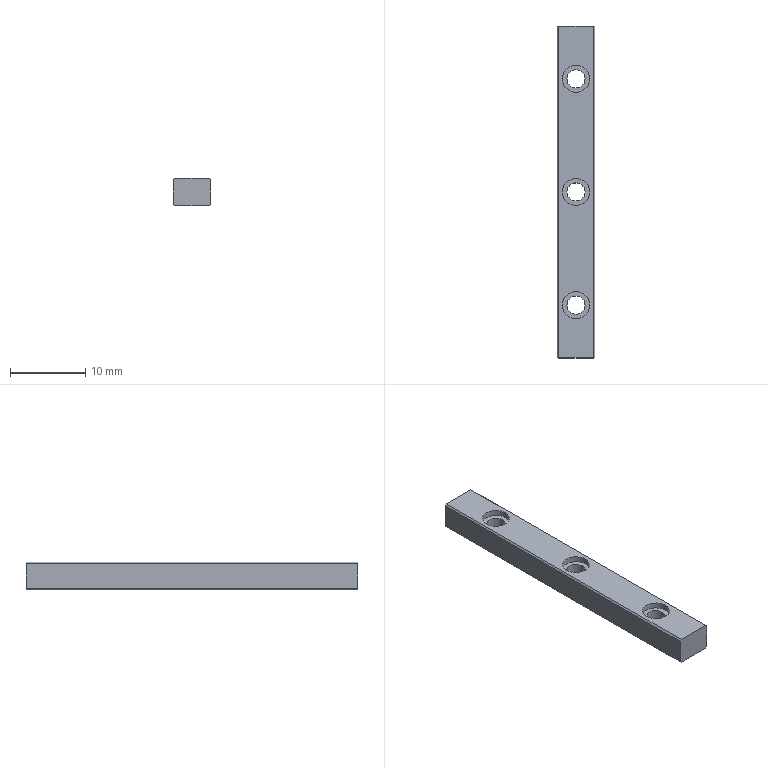Part | SolidWorks | features BaseBody 1 | 1 solid | 25 faces | box 5 x 44 x 3.7 mm | volume 746.693 mm3 | plane 13 | cylinder 12 | commonest cylinder face diameters 2.4 x6 3.6 x6
STEP:
#1=CARTESIAN_POINT('',(13.914,-6.044,0.));
#2=VERTEX_POINT('',#1);
#3=CARTESIAN_POINT('',(11.514,-6.044,0.));
#4=VERTEX_POINT('',#3);
#5=CARTESIAN_POINT('',(12.714,-6.044,0.));
#6=DIRECTION('',(0.,0.,-1.));
#7=DIRECTION('',(1.,0.,0.));
#8=AXIS2_PLACEMENT_3D('',#5,#6,#7);
#9=CIRCLE('',#8,1.2);
#10=EDGE_CURVE('',#2,#4,#9,.T.);
#11=ORIENTED_EDGE('',*,*,#10,.T.);
#12=CARTESIAN_POINT('',(11.514,-6.044,2.9));
#13=VERTEX_POINT('',#12);
#14=CARTESIAN_POINT('',(11.514,-6.044,-48.671));
#15=DIRECTION('',(0.,0.,1.));
#16=VECTOR('',#15,1000.);
#17=LINE('',#14,#16);
#18=EDGE_CURVE('',#4,#13,#17,.T.);
#19=ORIENTED_EDGE('',*,*,#18,.T.);
#20=CARTESIAN_POINT('',(13.914,-6.044,2.9));
#21=VERTEX_POINT('',#20);
#22=CARTESIAN_POINT('',(12.714,-6.044,2.9));
#23=DIRECTION('',(0.,0.,-1.));
#24=DIRECTION('',(1.,0.,0.));
#25=AXIS2_PLACEMENT_3D('',#22,#23,#24);
#26=CIRCLE('',#25,1.2);
#27=EDGE_CURVE('',#21,#13,#26,.T.);
#28=ORIENTED_EDGE('',*,*,#27,.F.);
#29=CARTESIAN_POINT('',(13.914,-6.044,-48.671));
#30=DIRECTION('',(0.,0.,1.));
#31=VECTOR('',#30,1000.);
#32=LINE('',#29,#31);
#33=EDGE_CURVE('',#2,#21,#32,.T.);
#34=ORIENTED_EDGE('',*,*,#33,.F.);
#35=EDGE_LOOP('',(#11,#19,#28,#34));
#36=FACE_OUTER_BOUND('',#35,.T.);
#37=CARTESIAN_POINT('',(12.714,-6.044,-48.671));
#38=DIRECTION('',(0.,0.,1.));
#39=DIRECTION('',(1.,0.,0.));
#40=AXIS2_PLACEMENT_3D('',#37,#38,#39);
#41=CYLINDRICAL_SURFACE('',#40,1.2);
#42=ADVANCED_FACE('',(#36),#41,.F.);
#43=CARTESIAN_POINT('',(13.914,-21.044,0.));
#44=VERTEX_POINT('',#43);
#45=CARTESIAN_POINT('',(11.514,-21.044,0.));
#46=VERTEX_POINT('',#45);
#47=CARTESIAN_POINT('',(12.714,-21.044,0.));
#48=DIRECTION('',(0.,0.,-1.));
#49=DIRECTION('',(1.,0.,0.));
#50=AXIS2_PLACEMENT_3D('',#47,#48,#49);
#51=CIRCLE('',#50,1.2);
#52=EDGE_CURVE('',#44,#46,#51,.T.);
#53=ORIENTED_EDGE('',*,*,#52,.T.);
#54=CARTESIAN_POINT('',(11.514,-21.044,2.9));
#55=VERTEX_POINT('',#54);
#56=CARTESIAN_POINT('',(11.514,-21.044,-48.671));
#57=DIRECTION('',(0.,0.,1.));
#58=VECTOR('',#57,1000.);
#59=LINE('',#56,#58);
#60=EDGE_CURVE('',#46,#55,#59,.T.);
#61=ORIENTED_EDGE('',*,*,#60,.T.);
#62=CARTESIAN_POINT('',(13.914,-21.044,2.9));
#63=VERTEX_POINT('',#62);
#64=CARTESIAN_POINT('',(12.714,-21.044,2.9));
#65=DIRECTION('',(0.,0.,-1.));
#66=DIRECTION('',(1.,0.,0.));
#67=AXIS2_PLACEMENT_3D('',#64,#65,#66);
#68=CIRCLE('',#67,1.2);
#69=EDGE_CURVE('',#63,#55,#68,.T.);
#70=ORIENTED_EDGE('',*,*,#69,.F.);
#71=CARTESIAN_POINT('',(13.914,-21.044,-48.671));
#72=DIRECTION('',(0.,0.,1.));
#73=VECTOR('',#72,1000.);
#74=LINE('',#71,#73);
#75=EDGE_CURVE('',#44,#63,#74,.T.);
#76=ORIENTED_EDGE('',*,*,#75,.F.);
#77=EDGE_LOOP('',(#53,#61,#70,#76));
#78=FACE_OUTER_BOUND('',#77,.T.);
#79=CARTESIAN_POINT('',(12.714,-21.044,-48.671));
#80=DIRECTION('',(0.,0.,1.));
#81=DIRECTION('',(1.,0.,0.));
#82=AXIS2_PLACEMENT_3D('',#79,#80,#81);
#83=CYLINDRICAL_SURFACE('',#82,1.2);
#84=ADVANCED_FACE('',(#78),#83,.F.);
#85=CARTESIAN_POINT('',(13.914,-36.044,0.));
#86=VERTEX_POINT('',#85);
#87=CARTESIAN_POINT('',(11.514,-36.044,0.));
#88=VERTEX_POINT('',#87);
#89=CARTESIAN_POINT('',(12.714,-36.044,0.));
#90=DIRECTION('',(0.,0.,-1.));
#91=DIRECTION('',(1.,0.,0.));
#92=AXIS2_PLACEMENT_3D('',#89,#90,#91);
#93=CIRCLE('',#92,1.2);
#94=EDGE_CURVE('',#86,#88,#93,.T.);
#95=ORIENTED_EDGE('',*,*,#94,.T.);
#96=CARTESIAN_POINT('',(11.514,-36.044,2.9));
#97=VERTEX_POINT('',#96);
#98=CARTESIAN_POINT('',(11.514,-36.044,-48.671));
#99=DIRECTION('',(0.,0.,1.));
#100=VECTOR('',#99,1000.);
#101=LINE('',#98,#100);
#102=EDGE_CURVE('',#88,#97,#101,.T.);
#103=ORIENTED_EDGE('',*,*,#102,.T.);
#104=CARTESIAN_POINT('',(13.914,-36.044,2.9));
#105=VERTEX_POINT('',#104);
#106=CARTESIAN_POINT('',(12.714,-36.044,2.9));
#107=DIRECTION('',(0.,0.,-1.));
#108=DIRECTION('',(1.,0.,0.));
#109=AXIS2_PLACEMENT_3D('',#106,#107,#108);
#110=CIRCLE('',#109,1.2);
#111=EDGE_CURVE('',#105,#97,#110,.T.);
#112=ORIENTED_EDGE('',*,*,#111,.F.);
#113=CARTESIAN_POINT('',(13.914,-36.044,-48.671));
#114=DIRECTION('',(0.,0.,1.));
#115=VECTOR('',#114,1000.);
#116=LINE('',#113,#115);
#117=EDGE_CURVE('',#86,#105,#116,.T.);
#118=ORIENTED_EDGE('',*,*,#117,.F.);
#119=EDGE_LOOP('',(#95,#103,#112,#118));
#120=FACE_OUTER_BOUND('',#119,.T.);
#121=CARTESIAN_POINT('',(12.714,-36.044,-48.671));
#122=DIRECTION('',(0.,0.,1.));
#123=DIRECTION('',(1.,0.,0.));
#124=AXIS2_PLACEMENT_3D('',#121,#122,#123);
#125=CYLINDRICAL_SURFACE('',#124,1.2);
#126=ADVANCED_FACE('',(#120),#125,.F.);
#127=CARTESIAN_POINT('',(10.914,-6.044,2.9));
#128=VERTEX_POINT('',#127);
#129=CARTESIAN_POINT('',(14.514,-6.044,2.9));
#130=VERTEX_POINT('',#129);
#131=CARTESIAN_POINT('',(12.714,-6.044,2.9));
#132=DIRECTION('',(0.,0.,1.));
#133=DIRECTION('',(1.,0.,0.));
#134=AXIS2_PLACEMENT_3D('',#131,#132,#133);
#135=CIRCLE('',#134,1.8);
#136=EDGE_CURVE('',#128,#130,#135,.T.);
#137=ORIENTED_EDGE('',*,*,#136,.F.);
#138=CARTESIAN_POINT('',(10.914,-6.044,3.7));
#139=VERTEX_POINT('',#138);
#140=CARTESIAN_POINT('',(10.914,-6.044,3.3));
#141=DIRECTION('',(0.,0.,1.));
#142=VECTOR('',#141,1000.);
#143=LINE('',#140,#142);
#144=EDGE_CURVE('',#128,#139,#143,.T.);
#145=ORIENTED_EDGE('',*,*,#144,.T.);
#146=CARTESIAN_POINT('',(14.514,-6.044,3.7));
#147=VERTEX_POINT('',#146);
#148=CARTESIAN_POINT('',(12.714,-6.044,3.7));
#149=DIRECTION('',(0.,0.,-1.));
#150=DIRECTION('',(1.,0.,0.));
#151=AXIS2_PLACEMENT_3D('',#148,#149,#150);
#152=CIRCLE('',#151,1.8);
#153=EDGE_CURVE('',#147,#139,#152,.T.);
#154=ORIENTED_EDGE('',*,*,#153,.F.);
#155=CARTESIAN_POINT('',(14.514,-6.044,3.3));
#156=DIRECTION('',(0.,0.,1.));
#157=VECTOR('',#156,1000.);
#158=LINE('',#155,#157);
#159=EDGE_CURVE('',#130,#147,#158,.T.);
#160=ORIENTED_EDGE('',*,*,#159,.F.);
#161=EDGE_LOOP('',(#137,#145,#154,#160));
#162=FACE_OUTER_BOUND('',#161,.T.);
#163=CARTESIAN_POINT('',(12.714,-6.044,3.3));
#164=DIRECTION('',(0.,0.,1.));
#165=DIRECTION('',(1.,0.,0.));
#166=AXIS2_PLACEMENT_3D('',#163,#164,#165);
#167=CYLINDRICAL_SURFACE('',#166,1.8);
#168=ADVANCED_FACE('',(#162),#167,.F.);
#169=CARTESIAN_POINT('',(10.914,-21.044,2.9));
#170=VERTEX_POINT('',#169);
#171=CARTESIAN_POINT('',(14.514,-21.044,2.9));
#172=VERTEX_POINT('',#171);
#173=CARTESIAN_POINT('',(12.714,-21.044,2.9));
#174=DIRECTION('',(0.,0.,1.));
#175=DIRECTION('',(1.,0.,0.));
#176=AXIS2_PLACEMENT_3D('',#173,#174,#175);
#177=CIRCLE('',#176,1.8);
#178=EDGE_CURVE('',#170,#172,#177,.T.);
#179=ORIENTED_EDGE('',*,*,#178,.F.);
#180=CARTESIAN_POINT('',(10.914,-21.044,3.7));
#181=VERTEX_POINT('',#180);
#182=CARTESIAN_POINT('',(10.914,-21.044,3.3));
#183=DIRECTION('',(0.,0.,1.));
#184=VECTOR('',#183,1000.);
#185=LINE('',#182,#184);
#186=EDGE_CURVE('',#170,#181,#185,.T.);
#187=ORIENTED_EDGE('',*,*,#186,.T.);
#188=CARTESIAN_POINT('',(14.514,-21.044,3.7));
#189=VERTEX_POINT('',#188);
#190=CARTESIAN_POINT('',(12.714,-21.044,3.7));
#191=DIRECTION('',(0.,0.,-1.));
#192=DIRECTION('',(1.,0.,0.));
#193=AXIS2_PLACEMENT_3D('',#190,#191,#192);
#194=CIRCLE('',#193,1.8);
#195=EDGE_CURVE('',#189,#181,#194,.T.);
#196=ORIENTED_EDGE('',*,*,#195,.F.);
#197=CARTESIAN_POINT('',(14.514,-21.044,3.3));
#198=DIRECTION('',(0.,0.,1.));
#199=VECTOR('',#198,1000.);
#200=LINE('',#197,#199);
#201=EDGE_CURVE('',#172,#189,#200,.T.);
#202=ORIENTED_EDGE('',*,*,#201,.F.);
#203=EDGE_LOOP('',(#179,#187,#196,#202));
#204=FACE_OUTER_BOUND('',#203,.T.);
#205=CARTESIAN_POINT('',(12.714,-21.044,3.3));
#206=DIRECTION('',(0.,0.,1.));
#207=DIRECTION('',(1.,0.,0.));
#208=AXIS2_PLACEMENT_3D('',#205,#206,#207);
#209=CYLINDRICAL_SURFACE('',#208,1.8);
#210=ADVANCED_FACE('',(#204),#209,.F.);
#211=CARTESIAN_POINT('',(10.914,-36.044,2.9));
#212=VERTEX_POINT('',#211);
#213=CARTESIAN_POINT('',(14.514,-36.044,2.9));
#214=VERTEX_POINT('',#213);
#215=CARTESIAN_POINT('',(12.714,-36.044,2.9));
#216=DIRECTION('',(0.,0.,1.));
#217=DIRECTION('',(1.,0.,0.));
#218=AXIS2_PLACEMENT_3D('',#215,#216,#217);
#219=CIRCLE('',#218,1.8);
#220=EDGE_CURVE('',#212,#214,#219,.T.);
#221=ORIENTED_EDGE('',*,*,#220,.F.);
#222=CARTESIAN_POINT('',(10.914,-36.044,3.7));
#223=VERTEX_POINT('',#222);
#224=CARTESIAN_POINT('',(10.914,-36.044,3.3));
#225=DIRECTION('',(0.,0.,1.));
#226=VECTOR('',#225,1000.);
#227=LINE('',#224,#226);
#228=EDGE_CURVE('',#212,#223,#227,.T.);
#229=ORIENTED_EDGE('',*,*,#228,.T.);
#230=CARTESIAN_POINT('',(14.514,-36.044,3.7));
#231=VERTEX_POINT('',#230);
#232=CARTESIAN_POINT('',(12.714,-36.044,3.7));
#233=DIRECTION('',(0.,0.,-1.));
#234=DIRECTION('',(1.,0.,0.));
#235=AXIS2_PLACEMENT_3D('',#232,#233,#234);
#236=CIRCLE('',#235,1.8);
#237=EDGE_CURVE('',#231,#223,#236,.T.);
#238=ORIENTED_EDGE('',*,*,#237,.F.);
#239=CARTESIAN_POINT('',(14.514,-36.044,3.3));
#240=DIRECTION('',(0.,0.,1.));
#241=VECTOR('',#240,1000.);
#242=LINE('',#239,#241);
#243=EDGE_CURVE('',#214,#231,#242,.T.);
#244=ORIENTED_EDGE('',*,*,#243,.F.);
#245=EDGE_LOOP('',(#221,#229,#238,#244));
#246=FACE_OUTER_BOUND('',#245,.T.);
#247=CARTESIAN_POINT('',(12.714,-36.044,3.3));
#248=DIRECTION('',(0.,0.,1.));
#249=DIRECTION('',(1.,0.,0.));
#250=AXIS2_PLACEMENT_3D('',#247,#248,#249);
#251=CYLINDRICAL_SURFACE('',#250,1.8);
#252=ADVANCED_FACE('',(#246),#251,.F.);
#253=ORIENTED_EDGE('',*,*,#10,.F.);
#254=CARTESIAN_POINT('',(12.714,-6.044,0.));
#255=DIRECTION('',(0.,0.,-1.));
#256=DIRECTION('',(1.,0.,0.));
#257=AXIS2_PLACEMENT_3D('',#254,#255,#256);
#258=CIRCLE('',#257,1.2);
#259=EDGE_CURVE('',#4,#2,#258,.T.);
#260=ORIENTED_EDGE('',*,*,#259,.F.);
#261=EDGE_LOOP('',(#253,#260));
#262=FACE_BOUND('',#261,.T.);
#263=ORIENTED_EDGE('',*,*,#52,.F.);
#264=CARTESIAN_POINT('',(12.714,-21.044,0.));
#265=DIRECTION('',(0.,0.,-1.));
#266=DIRECTION('',(1.,0.,0.));
#267=AXIS2_PLACEMENT_3D('',#264,#265,#266);
#268=CIRCLE('',#267,1.2);
#269=EDGE_CURVE('',#46,#44,#268,.T.);
#270=ORIENTED_EDGE('',*,*,#269,.F.);
#271=EDGE_LOOP('',(#263,#270));
#272=FACE_BOUND('',#271,.T.);
#273=ORIENTED_EDGE('',*,*,#94,.F.);
#274=CARTESIAN_POINT('',(12.714,-36.044,0.));
#275=DIRECTION('',(0.,0.,-1.));
#276=DIRECTION('',(1.,0.,0.));
#277=AXIS2_PLACEMENT_3D('',#274,#275,#276);
#278=CIRCLE('',#277,1.2);
#279=EDGE_CURVE('',#88,#86,#278,.T.);
#280=ORIENTED_EDGE('',*,*,#279,.F.);
#281=EDGE_LOOP('',(#273,#280));
#282=FACE_BOUND('',#281,.T.);
#283=CARTESIAN_POINT('',(10.414,-43.044,0.));
#284=VERTEX_POINT('',#283);
#285=CARTESIAN_POINT('',(15.014,-43.044,0.));
#286=VERTEX_POINT('',#285);
#287=CARTESIAN_POINT('',(12.714,-43.044,0.));
#288=DIRECTION('',(1.,0.,0.));
#289=VECTOR('',#288,1000.);
#290=LINE('',#287,#289);
#291=EDGE_CURVE('',#284,#286,#290,.T.);
#292=ORIENTED_EDGE('',*,*,#291,.F.);
#293=CARTESIAN_POINT('',(10.414,0.9558,0.));
#294=VERTEX_POINT('',#293);
#295=CARTESIAN_POINT('',(10.414,-21.044,0.));
#296=DIRECTION('',(0.,-1.,0.));
#297=VECTOR('',#296,1000.);
#298=LINE('',#295,#297);
#299=EDGE_CURVE('',#294,#284,#298,.T.);
#300=ORIENTED_EDGE('',*,*,#299,.F.);
#301=CARTESIAN_POINT('',(15.014,0.9558,0.));
#302=VERTEX_POINT('',#301);
#303=CARTESIAN_POINT('',(12.714,0.9558,0.));
#304=DIRECTION('',(-1.,0.,0.));
#305=VECTOR('',#304,1000.);
#306=LINE('',#303,#305);
#307=EDGE_CURVE('',#302,#294,#306,.T.);
#308=ORIENTED_EDGE('',*,*,#307,.F.);
#309=CARTESIAN_POINT('',(15.014,-21.044,0.));
#310=DIRECTION('',(0.,1.,0.));
#311=VECTOR('',#310,1000.);
#312=LINE('',#309,#311);
#313=EDGE_CURVE('',#286,#302,#312,.T.);
#314=ORIENTED_EDGE('',*,*,#313,.F.);
#315=EDGE_LOOP('',(#292,#300,#308,#314));
#316=FACE_OUTER_BOUND('',#315,.T.);
#317=CARTESIAN_POINT('',(12.714,-21.044,0.));
#318=DIRECTION('',(0.,0.,1.));
#319=DIRECTION('',(1.,0.,0.));
#320=AXIS2_PLACEMENT_3D('',#317,#318,#319);
#321=PLANE('',#320);
#322=ADVANCED_FACE('',(#262,#272,#282,#316),#321,.F.);
#323=ORIENTED_EDGE('',*,*,#18,.F.);
#324=ORIENTED_EDGE('',*,*,#259,.T.);
#325=ORIENTED_EDGE('',*,*,#33,.T.);
#326=CARTESIAN_POINT('',(12.714,-6.044,2.9));
#327=DIRECTION('',(0.,0.,-1.));
#328=DIRECTION('',(1.,0.,0.));
#329=AXIS2_PLACEMENT_3D('',#326,#327,#328);
#330=CIRCLE('',#329,1.2);
#331=EDGE_CURVE('',#13,#21,#330,.T.);
#332=ORIENTED_EDGE('',*,*,#331,.F.);
#333=EDGE_LOOP('',(#323,#324,#325,#332));
#334=FACE_OUTER_BOUND('',#333,.T.);
#335=CARTESIAN_POINT('',(12.714,-6.044,-48.671));
#336=DIRECTION('',(0.,0.,1.));
#337=DIRECTION('',(1.,0.,0.));
#338=AXIS2_PLACEMENT_3D('',#335,#336,#337);
#339=CYLINDRICAL_SURFACE('',#338,1.2);
#340=ADVANCED_FACE('',(#334),#339,.F.);
#341=ORIENTED_EDGE('',*,*,#60,.F.);
#342=ORIENTED_EDGE('',*,*,#269,.T.);
#343=ORIENTED_EDGE('',*,*,#75,.T.);
#344=CARTESIAN_POINT('',(12.714,-21.044,2.9));
#345=DIRECTION('',(0.,0.,-1.));
#346=DIRECTION('',(1.,0.,0.));
#347=AXIS2_PLACEMENT_3D('',#344,#345,#346);
#348=CIRCLE('',#347,1.2);
#349=EDGE_CURVE('',#55,#63,#348,.T.);
#350=ORIENTED_EDGE('',*,*,#349,.F.);
#351=EDGE_LOOP('',(#341,#342,#343,#350));
#352=FACE_OUTER_BOUND('',#351,.T.);
#353=CARTESIAN_POINT('',(12.714,-21.044,-48.671));
#354=DIRECTION('',(0.,0.,1.));
#355=DIRECTION('',(1.,0.,0.));
#356=AXIS2_PLACEMENT_3D('',#353,#354,#355);
#357=CYLINDRICAL_SURFACE('',#356,1.2);
#358=ADVANCED_FACE('',(#352),#357,.F.);
#359=ORIENTED_EDGE('',*,*,#102,.F.);
#360=ORIENTED_EDGE('',*,*,#279,.T.);
#361=ORIENTED_EDGE('',*,*,#117,.T.);
#362=CARTESIAN_POINT('',(12.714,-36.044,2.9));
#363=DIRECTION('',(0.,0.,-1.));
#364=DIRECTION('',(1.,0.,0.));
#365=AXIS2_PLACEMENT_3D('',#362,#363,#364);
#366=CIRCLE('',#365,1.2);
#367=EDGE_CURVE('',#97,#105,#366,.T.);
#368=ORIENTED_EDGE('',*,*,#367,.F.);
#369=EDGE_LOOP('',(#359,#360,#361,#368));
#370=FACE_OUTER_BOUND('',#369,.T.);
#371=CARTESIAN_POINT('',(12.714,-36.044,-48.671));
#372=DIRECTION('',(0.,0.,1.));
#373=DIRECTION('',(1.,0.,0.));
#374=AXIS2_PLACEMENT_3D('',#371,#372,#373);
#375=CYLINDRICAL_SURFACE('',#374,1.2);
#376=ADVANCED_FACE('',(#370),#375,.F.);
#377=CARTESIAN_POINT('',(15.214,0.9558,0.2));
#378=VERTEX_POINT('',#377);
#379=CARTESIAN_POINT('',(15.114,0.9558,0.1));
#380=DIRECTION('',(0.7071,0.,0.7071));
#381=VECTOR('',#380,1000.);
#382=LINE('',#379,#381);
#383=EDGE_CURVE('',#302,#378,#382,.T.);
#384=ORIENTED_EDGE('',*,*,#383,.T.);
#385=CARTESIAN_POINT('',(15.214,-43.044,0.2));
#386=VERTEX_POINT('',#385);
#387=CARTESIAN_POINT('',(15.214,-10.044,0.2));
#388=DIRECTION('',(0.,-1.,0.));
#389=VECTOR('',#388,1000.);
#390=LINE('',#387,#389);
#391=EDGE_CURVE('',#378,#386,#390,.T.);
#392=ORIENTED_EDGE('',*,*,#391,.T.);
#393=CARTESIAN_POINT('',(15.114,-43.044,0.1));
#394=DIRECTION('',(-0.7071,0.,-0.7071));
#395=VECTOR('',#394,1000.);
#396=LINE('',#393,#395);
#397=EDGE_CURVE('',#386,#286,#396,.T.);
#398=ORIENTED_EDGE('',*,*,#397,.T.);
#399=ORIENTED_EDGE('',*,*,#313,.T.);
#400=EDGE_LOOP('',(#384,#392,#398,#399));
#401=FACE_OUTER_BOUND('',#400,.T.);
#402=CARTESIAN_POINT('',(15.114,-10.044,0.1));
#403=DIRECTION('',(0.7071,0.,-0.7071));
#404=DIRECTION('',(-0.7071,0.,-0.7071));
#405=AXIS2_PLACEMENT_3D('',#402,#403,#404);
#406=PLANE('',#405);
#407=ADVANCED_FACE('',(#401),#406,.T.);
#408=CARTESIAN_POINT('',(10.214,-43.044,0.2));
#409=VERTEX_POINT('',#408);
#410=CARTESIAN_POINT('',(10.214,-43.044,0.2));
#411=DIRECTION('',(0.7071,0.,-0.7071));
#412=VECTOR('',#411,1000.);
#413=LINE('',#410,#412);
#414=EDGE_CURVE('',#409,#284,#413,.T.);
#415=ORIENTED_EDGE('',*,*,#414,.T.);
#416=ORIENTED_EDGE('',*,*,#291,.T.);
#417=ORIENTED_EDGE('',*,*,#397,.F.);
#418=CARTESIAN_POINT('',(15.214,-43.044,3.5));
#419=VERTEX_POINT('',#418);
#420=CARTESIAN_POINT('',(15.214,-43.044,0.));
#421=DIRECTION('',(0.,0.,1.));
#422=VECTOR('',#421,1000.);
#423=LINE('',#420,#422);
#424=EDGE_CURVE('',#386,#419,#423,.T.);
#425=ORIENTED_EDGE('',*,*,#424,.T.);
#426=CARTESIAN_POINT('',(15.014,-43.044,3.7));
#427=VERTEX_POINT('',#426);
#428=CARTESIAN_POINT('',(15.114,-43.044,3.6));
#429=DIRECTION('',(0.7071,0.,-0.7071));
#430=VECTOR('',#429,1000.);
#431=LINE('',#428,#430);
#432=EDGE_CURVE('',#427,#419,#431,.T.);
#433=ORIENTED_EDGE('',*,*,#432,.F.);
#434=CARTESIAN_POINT('',(10.414,-43.044,3.7));
#435=VERTEX_POINT('',#434);
#436=CARTESIAN_POINT('',(15.214,-43.044,3.7));
#437=DIRECTION('',(-1.,0.,0.));
#438=VECTOR('',#437,1000.);
#439=LINE('',#436,#438);
#440=EDGE_CURVE('',#427,#435,#439,.T.);
#441=ORIENTED_EDGE('',*,*,#440,.T.);
#442=CARTESIAN_POINT('',(10.214,-43.044,3.5));
#443=VERTEX_POINT('',#442);
#444=CARTESIAN_POINT('',(10.314,-43.044,3.6));
#445=DIRECTION('',(0.7071,0.,0.7071));
#446=VECTOR('',#445,1000.);
#447=LINE('',#444,#446);
#448=EDGE_CURVE('',#443,#435,#447,.T.);
#449=ORIENTED_EDGE('',*,*,#448,.F.);
#450=CARTESIAN_POINT('',(10.214,-43.044,0.));
#451=DIRECTION('',(0.,0.,-1.));
#452=VECTOR('',#451,1000.);
#453=LINE('',#450,#452);
#454=EDGE_CURVE('',#443,#409,#453,.T.);
#455=ORIENTED_EDGE('',*,*,#454,.T.);
#456=EDGE_LOOP('',(#415,#416,#417,#425,#433,#441,#449,#455));
#457=FACE_OUTER_BOUND('',#456,.T.);
#458=CARTESIAN_POINT('',(15.214,-43.044,0.));
#459=DIRECTION('',(0.,-1.,0.));
#460=DIRECTION('',(0.,0.,-1.));
#461=AXIS2_PLACEMENT_3D('',#458,#459,#460);
#462=PLANE('',#461);
#463=ADVANCED_FACE('',(#457),#462,.T.);
#464=ORIENTED_EDGE('',*,*,#414,.F.);
#465=CARTESIAN_POINT('',(10.214,0.9558,0.2));
#466=VERTEX_POINT('',#465);
#467=CARTESIAN_POINT('',(10.214,-32.044,0.2));
#468=DIRECTION('',(0.,1.,0.));
#469=VECTOR('',#468,1000.);
#470=LINE('',#467,#469);
#471=EDGE_CURVE('',#409,#466,#470,.T.);
#472=ORIENTED_EDGE('',*,*,#471,.T.);
#473=CARTESIAN_POINT('',(10.314,0.9558,0.1));
#474=DIRECTION('',(0.7071,0.,-0.7071));
#475=VECTOR('',#474,1000.);
#476=LINE('',#473,#475);
#477=EDGE_CURVE('',#466,#294,#476,.T.);
#478=ORIENTED_EDGE('',*,*,#477,.T.);
#479=ORIENTED_EDGE('',*,*,#299,.T.);
#480=EDGE_LOOP('',(#464,#472,#478,#479));
#481=FACE_OUTER_BOUND('',#480,.T.);
#482=CARTESIAN_POINT('',(10.314,-32.044,0.1));
#483=DIRECTION('',(-0.7071,0.,-0.7071));
#484=DIRECTION('',(-0.7071,0.,0.7071));
#485=AXIS2_PLACEMENT_3D('',#482,#483,#484);
#486=PLANE('',#485);
#487=ADVANCED_FACE('',(#481),#486,.T.);
#488=CARTESIAN_POINT('',(15.214,0.9558,3.5));
#489=VERTEX_POINT('',#488);
#490=CARTESIAN_POINT('',(15.014,0.9558,3.7));
#491=VERTEX_POINT('',#490);
#492=CARTESIAN_POINT('',(15.114,0.9558,3.6));
#493=DIRECTION('',(-0.7071,0.,0.7071));
#494=VECTOR('',#493,1000.);
#495=LINE('',#492,#494);
#496=EDGE_CURVE('',#489,#491,#495,.T.);
#497=ORIENTED_EDGE('',*,*,#496,.F.);
#498=CARTESIAN_POINT('',(15.214,0.9558,0.));
#499=DIRECTION('',(0.,0.,-1.));
#500=VECTOR('',#499,1000.);
#501=LINE('',#498,#500);
#502=EDGE_CURVE('',#489,#378,#501,.T.);
#503=ORIENTED_EDGE('',*,*,#502,.T.);
#504=ORIENTED_EDGE('',*,*,#383,.F.);
#505=ORIENTED_EDGE('',*,*,#307,.T.);
#506=ORIENTED_EDGE('',*,*,#477,.F.);
#507=CARTESIAN_POINT('',(10.214,0.9558,3.5));
#508=VERTEX_POINT('',#507);
#509=CARTESIAN_POINT('',(10.214,0.9558,0.));
#510=DIRECTION('',(0.,0.,1.));
#511=VECTOR('',#510,1000.);
#512=LINE('',#509,#511);
#513=EDGE_CURVE('',#466,#508,#512,.T.);
#514=ORIENTED_EDGE('',*,*,#513,.T.);
#515=CARTESIAN_POINT('',(10.414,0.9558,3.7));
#516=VERTEX_POINT('',#515);
#517=CARTESIAN_POINT('',(10.314,0.9558,3.6));
#518=DIRECTION('',(-0.7071,0.,-0.7071));
#519=VECTOR('',#518,1000.);
#520=LINE('',#517,#519);
#521=EDGE_CURVE('',#516,#508,#520,.T.);
#522=ORIENTED_EDGE('',*,*,#521,.F.);
#523=CARTESIAN_POINT('',(10.214,0.9558,3.7));
#524=DIRECTION('',(1.,0.,0.));
#525=VECTOR('',#524,1000.);
#526=LINE('',#523,#525);
#527=EDGE_CURVE('',#516,#491,#526,.T.);
#528=ORIENTED_EDGE('',*,*,#527,.T.);
#529=EDGE_LOOP('',(#497,#503,#504,#505,#506,#514,#522,#528));
#530=FACE_OUTER_BOUND('',#529,.T.);
#531=CARTESIAN_POINT('',(10.214,0.9558,0.));
#532=DIRECTION('',(0.,1.,0.));
#533=DIRECTION('',(0.,0.,1.));
#534=AXIS2_PLACEMENT_3D('',#531,#532,#533);
#535=PLANE('',#534);
#536=ADVANCED_FACE('',(#530),#535,.T.);
#537=ORIENTED_EDGE('',*,*,#27,.T.);
#538=ORIENTED_EDGE('',*,*,#331,.T.);
#539=EDGE_LOOP('',(#537,#538));
#540=FACE_BOUND('',#539,.T.);
#541=CARTESIAN_POINT('',(12.714,-6.044,2.9));
#542=DIRECTION('',(0.,0.,1.));
#543=DIRECTION('',(1.,0.,0.));
#544=AXIS2_PLACEMENT_3D('',#541,#542,#543);
#545=CIRCLE('',#544,1.8);
#546=EDGE_CURVE('',#130,#128,#545,.T.);
#547=ORIENTED_EDGE('',*,*,#546,.T.);
#548=ORIENTED_EDGE('',*,*,#136,.T.);
#549=EDGE_LOOP('',(#547,#548));
#550=FACE_OUTER_BOUND('',#549,.T.);
#551=CARTESIAN_POINT('',(12.714,-6.044,2.9));
#552=DIRECTION('',(0.,0.,1.));
#553=DIRECTION('',(1.,0.,0.));
#554=AXIS2_PLACEMENT_3D('',#551,#552,#553);
#555=PLANE('',#554);
#556=ADVANCED_FACE('',(#540,#550),#555,.T.);
#557=ORIENTED_EDGE('',*,*,#69,.T.);
#558=ORIENTED_EDGE('',*,*,#349,.T.);
#559=EDGE_LOOP('',(#557,#558));
#560=FACE_BOUND('',#559,.T.);
#561=CARTESIAN_POINT('',(12.714,-21.044,2.9));
#562=DIRECTION('',(0.,0.,1.));
#563=DIRECTION('',(1.,0.,0.));
#564=AXIS2_PLACEMENT_3D('',#561,#562,#563);
#565=CIRCLE('',#564,1.8);
#566=EDGE_CURVE('',#172,#170,#565,.T.);
#567=ORIENTED_EDGE('',*,*,#566,.T.);
#568=ORIENTED_EDGE('',*,*,#178,.T.);
#569=EDGE_LOOP('',(#567,#568));
#570=FACE_OUTER_BOUND('',#569,.T.);
#571=CARTESIAN_POINT('',(12.714,-21.044,2.9));
#572=DIRECTION('',(0.,0.,1.));
#573=DIRECTION('',(1.,0.,0.));
#574=AXIS2_PLACEMENT_3D('',#571,#572,#573);
#575=PLANE('',#574);
#576=ADVANCED_FACE('',(#560,#570),#575,.T.);
#577=ORIENTED_EDGE('',*,*,#111,.T.);
#578=ORIENTED_EDGE('',*,*,#367,.T.);
#579=EDGE_LOOP('',(#577,#578));
#580=FACE_BOUND('',#579,.T.);
#581=CARTESIAN_POINT('',(12.714,-36.044,2.9));
#582=DIRECTION('',(0.,0.,1.));
#583=DIRECTION('',(1.,0.,0.));
#584=AXIS2_PLACEMENT_3D('',#581,#582,#583);
#585=CIRCLE('',#584,1.8);
#586=EDGE_CURVE('',#214,#212,#585,.T.);
#587=ORIENTED_EDGE('',*,*,#586,.T.);
#588=ORIENTED_EDGE('',*,*,#220,.T.);
#589=EDGE_LOOP('',(#587,#588));
#590=FACE_OUTER_BOUND('',#589,.T.);
#591=CARTESIAN_POINT('',(12.714,-36.044,2.9));
#592=DIRECTION('',(0.,0.,1.));
#593=DIRECTION('',(1.,0.,0.));
#594=AXIS2_PLACEMENT_3D('',#591,#592,#593);
#595=PLANE('',#594);
#596=ADVANCED_FACE('',(#580,#590),#595,.T.);
#597=CARTESIAN_POINT('',(15.214,0.9558,3.5));
#598=DIRECTION('',(0.,-1.,0.));
#599=VECTOR('',#598,1000.);
#600=LINE('',#597,#599);
#601=EDGE_CURVE('',#489,#419,#600,.T.);
#602=ORIENTED_EDGE('',*,*,#601,.T.);
#603=ORIENTED_EDGE('',*,*,#424,.F.);
#604=ORIENTED_EDGE('',*,*,#391,.F.);
#605=ORIENTED_EDGE('',*,*,#502,.F.);
#606=EDGE_LOOP('',(#602,#603,#604,#605));
#607=FACE_OUTER_BOUND('',#606,.T.);
#608=CARTESIAN_POINT('',(15.214,0.9558,0.));
#609=DIRECTION('',(1.,0.,0.));
#610=DIRECTION('',(0.,0.,-1.));
#611=AXIS2_PLACEMENT_3D('',#608,#609,#610);
#612=PLANE('',#611);
#613=ADVANCED_FACE('',(#607),#612,.T.);
#614=CARTESIAN_POINT('',(10.214,-43.044,3.5));
#615=DIRECTION('',(0.,1.,0.));
#616=VECTOR('',#615,1000.);
#617=LINE('',#614,#616);
#618=EDGE_CURVE('',#443,#508,#617,.T.);
#619=ORIENTED_EDGE('',*,*,#618,.T.);
#620=ORIENTED_EDGE('',*,*,#513,.F.);
#621=ORIENTED_EDGE('',*,*,#471,.F.);
#622=ORIENTED_EDGE('',*,*,#454,.F.);
#623=EDGE_LOOP('',(#619,#620,#621,#622));
#624=FACE_OUTER_BOUND('',#623,.T.);
#625=CARTESIAN_POINT('',(10.214,-43.044,0.));
#626=DIRECTION('',(-1.,0.,0.));
#627=DIRECTION('',(0.,0.,1.));
#628=AXIS2_PLACEMENT_3D('',#625,#626,#627);
#629=PLANE('',#628);
#630=ADVANCED_FACE('',(#624),#629,.T.);
#631=ORIENTED_EDGE('',*,*,#153,.T.);
#632=CARTESIAN_POINT('',(12.714,-6.044,3.7));
#633=DIRECTION('',(0.,0.,-1.));
#634=DIRECTION('',(1.,0.,0.));
#635=AXIS2_PLACEMENT_3D('',#632,#633,#634);
#636=CIRCLE('',#635,1.8);
#637=EDGE_CURVE('',#139,#147,#636,.T.);
#638=ORIENTED_EDGE('',*,*,#637,.T.);
#639=EDGE_LOOP('',(#631,#638));
#640=FACE_BOUND('',#639,.T.);
#641=ORIENTED_EDGE('',*,*,#195,.T.);
#642=CARTESIAN_POINT('',(12.714,-21.044,3.7));
#643=DIRECTION('',(0.,0.,-1.));
#644=DIRECTION('',(1.,0.,0.));
#645=AXIS2_PLACEMENT_3D('',#642,#643,#644);
#646=CIRCLE('',#645,1.8);
#647=EDGE_CURVE('',#181,#189,#646,.T.);
#648=ORIENTED_EDGE('',*,*,#647,.T.);
#649=EDGE_LOOP('',(#641,#648));
#650=FACE_BOUND('',#649,.T.);
#651=ORIENTED_EDGE('',*,*,#237,.T.);
#652=CARTESIAN_POINT('',(12.714,-36.044,3.7));
#653=DIRECTION('',(0.,0.,-1.));
#654=DIRECTION('',(1.,0.,0.));
#655=AXIS2_PLACEMENT_3D('',#652,#653,#654);
#656=CIRCLE('',#655,1.8);
#657=EDGE_CURVE('',#223,#231,#656,.T.);
#658=ORIENTED_EDGE('',*,*,#657,.T.);
#659=EDGE_LOOP('',(#651,#658));
#660=FACE_BOUND('',#659,.T.);
#661=CARTESIAN_POINT('',(15.014,-21.044,3.7));
#662=DIRECTION('',(0.,1.,0.));
#663=VECTOR('',#662,1000.);
#664=LINE('',#661,#663);
#665=EDGE_CURVE('',#427,#491,#664,.T.);
#666=ORIENTED_EDGE('',*,*,#665,.T.);
#667=ORIENTED_EDGE('',*,*,#527,.F.);
#668=CARTESIAN_POINT('',(10.414,-21.044,3.7));
#669=DIRECTION('',(0.,-1.,0.));
#670=VECTOR('',#669,1000.);
#671=LINE('',#668,#670);
#672=EDGE_CURVE('',#516,#435,#671,.T.);
#673=ORIENTED_EDGE('',*,*,#672,.T.);
#674=ORIENTED_EDGE('',*,*,#440,.F.);
#675=EDGE_LOOP('',(#666,#667,#673,#674));
#676=FACE_OUTER_BOUND('',#675,.T.);
#677=CARTESIAN_POINT('',(12.714,-21.044,3.7));
#678=DIRECTION('',(0.,0.,1.));
#679=DIRECTION('',(1.,0.,0.));
#680=AXIS2_PLACEMENT_3D('',#677,#678,#679);
#681=PLANE('',#680);
#682=ADVANCED_FACE('',(#640,#650,#660,#676),#681,.T.);
#683=ORIENTED_EDGE('',*,*,#144,.F.);
#684=ORIENTED_EDGE('',*,*,#546,.F.);
#685=ORIENTED_EDGE('',*,*,#159,.T.);
#686=ORIENTED_EDGE('',*,*,#637,.F.);
#687=EDGE_LOOP('',(#683,#684,#685,#686));
#688=FACE_OUTER_BOUND('',#687,.T.);
#689=CARTESIAN_POINT('',(12.714,-6.044,3.3));
#690=DIRECTION('',(0.,0.,1.));
#691=DIRECTION('',(1.,0.,0.));
#692=AXIS2_PLACEMENT_3D('',#689,#690,#691);
#693=CYLINDRICAL_SURFACE('',#692,1.8);
#694=ADVANCED_FACE('',(#688),#693,.F.);
#695=ORIENTED_EDGE('',*,*,#186,.F.);
#696=ORIENTED_EDGE('',*,*,#566,.F.);
#697=ORIENTED_EDGE('',*,*,#201,.T.);
#698=ORIENTED_EDGE('',*,*,#647,.F.);
#699=EDGE_LOOP('',(#695,#696,#697,#698));
#700=FACE_OUTER_BOUND('',#699,.T.);
#701=CARTESIAN_POINT('',(12.714,-21.044,3.3));
#702=DIRECTION('',(0.,0.,1.));
#703=DIRECTION('',(1.,0.,0.));
#704=AXIS2_PLACEMENT_3D('',#701,#702,#703);
#705=CYLINDRICAL_SURFACE('',#704,1.8);
#706=ADVANCED_FACE('',(#700),#705,.F.);
#707=ORIENTED_EDGE('',*,*,#228,.F.);
#708=ORIENTED_EDGE('',*,*,#586,.F.);
#709=ORIENTED_EDGE('',*,*,#243,.T.);
#710=ORIENTED_EDGE('',*,*,#657,.F.);
#711=EDGE_LOOP('',(#707,#708,#709,#710));
#712=FACE_OUTER_BOUND('',#711,.T.);
#713=CARTESIAN_POINT('',(12.714,-36.044,3.3));
#714=DIRECTION('',(0.,0.,1.));
#715=DIRECTION('',(1.,0.,0.));
#716=AXIS2_PLACEMENT_3D('',#713,#714,#715);
#717=CYLINDRICAL_SURFACE('',#716,1.8);
#718=ADVANCED_FACE('',(#712),#717,.F.);
#719=ORIENTED_EDGE('',*,*,#496,.T.);
#720=ORIENTED_EDGE('',*,*,#665,.F.);
#721=ORIENTED_EDGE('',*,*,#432,.T.);
#722=ORIENTED_EDGE('',*,*,#601,.F.);
#723=EDGE_LOOP('',(#719,#720,#721,#722));
#724=FACE_OUTER_BOUND('',#723,.T.);
#725=CARTESIAN_POINT('',(15.114,-10.044,3.6));
#726=DIRECTION('',(0.7071,0.,0.7071));
#727=DIRECTION('',(0.7071,0.,-0.7071));
#728=AXIS2_PLACEMENT_3D('',#725,#726,#727);
#729=PLANE('',#728);
#730=ADVANCED_FACE('',(#724),#729,.T.);
#731=ORIENTED_EDGE('',*,*,#448,.T.);
#732=ORIENTED_EDGE('',*,*,#672,.F.);
#733=ORIENTED_EDGE('',*,*,#521,.T.);
#734=ORIENTED_EDGE('',*,*,#618,.F.);
#735=EDGE_LOOP('',(#731,#732,#733,#734));
#736=FACE_OUTER_BOUND('',#735,.T.);
#737=CARTESIAN_POINT('',(10.314,-32.044,3.6));
#738=DIRECTION('',(-0.7071,0.,0.7071));
#739=DIRECTION('',(0.7071,0.,0.7071));
#740=AXIS2_PLACEMENT_3D('',#737,#738,#739);
#741=PLANE('',#740);
#742=ADVANCED_FACE('',(#736),#741,.T.);
#743=CLOSED_SHELL('',(#42,#84,#126,#168,#210,#252,#322,#340,#358,#376,#407,#463,#487,#536,#556,#576,#596,#613,#630,#682,#694,#706,#718,#730,#742));
#744=MANIFOLD_SOLID_BREP('',#743);
#745=CARTESIAN_POINT('',(0.,0.,0.));
#746=DIRECTION('',(0.,0.,1.));
#747=DIRECTION('',(1.,0.,0.));
#748=AXIS2_PLACEMENT_3D('',#745,#746,#747);
#749=(LENGTH_UNIT()NAMED_UNIT(*)SI_UNIT(.MILLI.,.METRE.));
#750=UNCERTAINTY_MEASURE_WITH_UNIT(LENGTH_MEASURE(0.00001),#749,'','');
#751=(NAMED_UNIT(*)PLANE_ANGLE_UNIT()SI_UNIT($,.RADIAN.));
#752=(NAMED_UNIT(*)SI_UNIT($,.STERADIAN.)SOLID_ANGLE_UNIT());
#753=(GEOMETRIC_REPRESENTATION_CONTEXT(3)GLOBAL_UNCERTAINTY_ASSIGNED_CONTEXT((#750))GLOBAL_UNIT_ASSIGNED_CONTEXT((#749,#751,#752))REPRESENTATION_CONTEXT('',''));
#754=ADVANCED_BREP_SHAPE_REPRESENTATION('',(#744,#748),#753);